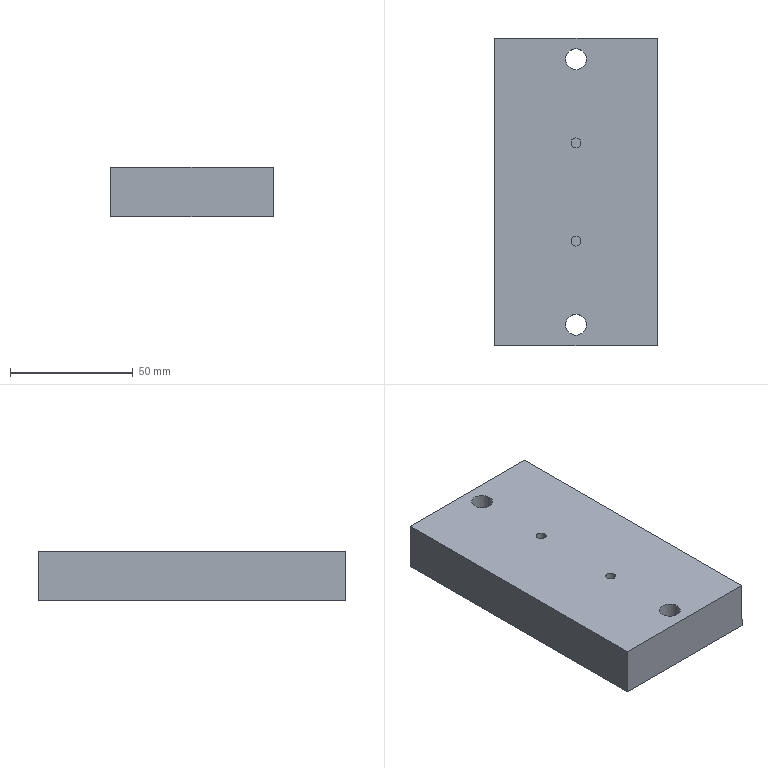NC program | NX | posted with a generic post | part box 65.936 x 125 x 20 mm
Lines 1209 to 2027 of 29196:
(PLANAR_MILL_1 , TOOL : D3R0)
N2308 T07 M6
N2310 G54
N2312 G17 G0 G90 X-29.604 Y-6.011 S5000 M3
N2314 G43 Z26.573 H7
N2316 G94 G1 Z-3.127 F5000.
N2318 X-29.572 Y-5.956 Z-3.128 F1000.
N2320 X-29.545 Y-5.795 Z-3.131
N2322 X-29.577 Y-5.636 Z-3.134
N2324 X-29.644 Y-5.519 Z-3.136
N2326 X-29.766 Y-5.412 Z-3.139
N2328 X-29.919 Y-5.355 Z-3.142
N2330 X-30.081 Z-3.145
N2332 X-30.234 Y-5.412 Z-3.148
N2334 X-30.356 Y-5.519 Z-3.151
N2336 X-30.423 Y-5.636 Z-3.153
N2338 X-30.45 Y-5.735 Z-3.155
N2340 Y-5.87 Z-3.157
N2342 X-30.406 Y-6.007 Z-3.16
N2344 X-30.322 Y-6.124 Z-3.162
N2346 X-30.205 Y-6.209 Z-3.165
N2348 X-30.067 Y-6.252 Z-3.167
N2350 X-29.933 Z-3.169
N2352 X-29.779 Y-6.2 Z-3.172
N2354 X-29.653 Y-6.097 Z-3.175
N2356 X-29.572 Y-5.956 Z-3.178
N2358 X-29.545 Y-5.795 Z-3.181
N2360 X-29.577 Y-5.636 Z-3.184
N2362 X-29.644 Y-5.519 Z-3.186
N2364 X-29.766 Y-5.412 Z-3.189
N2366 X-29.919 Y-5.355 Z-3.192
N2368 X-30.081 Z-3.195
N2370 X-30.234 Y-5.412 Z-3.197
N2372 X-30.356 Y-5.519 Z-3.2
N2374 X-30.423 Y-5.636 Z-3.203
N2376 X-30.45 Y-5.735 Z-3.204
N2378 Y-5.87 Z-3.207
N2380 X-30.406 Y-6.007 Z-3.209
N2382 X-30.322 Y-6.124 Z-3.212
N2384 X-30.205 Y-6.209 Z-3.214
N2386 X-30.067 Y-6.252 Z-3.217
N2388 X-29.933 Z-3.219
N2390 X-29.779 Y-6.2 Z-3.222
N2392 X-29.653 Y-6.097 Z-3.225
N2394 X-29.572 Y-5.956 Z-3.228
N2396 X-29.545 Y-5.795 Z-3.23
N2398 X-29.577 Y-5.636 Z-3.233
N2400 X-29.644 Y-5.519 Z-3.236
N2402 X-29.766 Y-5.412 Z-3.238
N2404 X-29.919 Y-5.355 Z-3.241
N2406 X-30.081 Z-3.244
N2408 X-30.234 Y-5.412 Z-3.247
N2410 X-30.356 Y-5.519 Z-3.25
N2412 X-30.423 Y-5.636 Z-3.252
N2414 X-30.45 Y-5.735 Z-3.254
N2416 Y-5.87 Z-3.256
N2418 X-30.406 Y-6.007 Z-3.259
N2420 X-30.322 Y-6.124 Z-3.261
N2422 X-30.205 Y-6.209 Z-3.264
N2424 X-30.067 Y-6.252 Z-3.266
N2426 X-29.933 Z-3.269
N2428 X-29.779 Y-6.2 Z-3.272
N2430 X-29.653 Y-6.097 Z-3.274
N2432 X-29.572 Y-5.956 Z-3.277
N2434 X-29.545 Y-5.795 Z-3.28
N2436 X-29.577 Y-5.636 Z-3.283
N2438 X-29.644 Y-5.519 Z-3.285
N2440 X-29.766 Y-5.412 Z-3.288
N2442 X-29.919 Y-5.355 Z-3.291
N2444 X-30.081 Z-3.294
N2446 X-30.234 Y-5.412 Z-3.297
N2448 X-30.356 Y-5.519 Z-3.3
N2450 X-30.423 Y-5.636 Z-3.302
N2452 X-30.45 Y-5.735 Z-3.304
N2454 Y-5.87 Z-3.306
N2456 X-30.406 Y-6.007 Z-3.309
N2458 X-30.322 Y-6.124 Z-3.311
N2460 X-30.205 Y-6.209 Z-3.314
N2462 X-30.067 Y-6.252 Z-3.316
N2464 X-29.933 Z-3.318
N2466 X-29.779 Y-6.2 Z-3.321
N2468 X-29.653 Y-6.097 Z-3.324
N2470 X-29.572 Y-5.956 Z-3.327
N2472 X-29.545 Y-5.795 Z-3.33
N2474 X-29.577 Y-5.636 Z-3.333
N2476 X-29.644 Y-5.519 Z-3.335
N2478 X-29.766 Y-5.412 Z-3.338
N2480 X-29.919 Y-5.355 Z-3.341
N2482 X-30.081 Z-3.344
N2484 X-30.234 Y-5.412 Z-3.346
N2486 X-30.356 Y-5.519 Z-3.349
N2488 X-30.423 Y-5.636 Z-3.352
N2490 X-30.45 Y-5.735 Z-3.353
N2492 Y-5.87 Z-3.356
N2494 X-30.406 Y-6.007 Z-3.358
N2496 X-30.322 Y-6.124 Z-3.361
N2498 X-30.205 Y-6.209 Z-3.363
N2500 X-30.067 Y-6.252 Z-3.366
N2502 X-29.933 Z-3.368
N2504 X-29.779 Y-6.2 Z-3.371
N2506 X-29.653 Y-6.097 Z-3.374
N2508 X-29.572 Y-5.956 Z-3.377
N2510 X-29.545 Y-5.795 Z-3.379
N2512 X-29.577 Y-5.636 Z-3.382
N2514 X-29.644 Y-5.519 Z-3.385
N2516 X-29.766 Y-5.412 Z-3.387
N2518 X-29.919 Y-5.355 Z-3.39
N2520 X-30.081 Z-3.393
N2522 X-30.234 Y-5.412 Z-3.396
N2524 X-30.356 Y-5.519 Z-3.399
N2526 X-30.423 Y-5.636 Z-3.401
N2528 X-30.45 Y-5.735 Z-3.403
N2530 Y-5.87 Z-3.405
N2532 X-30.406 Y-6.007 Z-3.408
N2534 X-30.322 Y-6.124 Z-3.41
N2536 X-30.205 Y-6.209 Z-3.413
N2538 X-30.067 Y-6.252 Z-3.415
N2540 X-29.933 Z-3.418
N2542 X-29.779 Y-6.2 Z-3.421
N2544 X-29.653 Y-6.097 Z-3.423
N2546 X-29.572 Y-5.956 Z-3.426
N2548 X-29.545 Y-5.795 Z-3.429
N2550 X-29.577 Y-5.636 Z-3.432
N2552 X-29.644 Y-5.519 Z-3.434
N2554 X-29.766 Y-5.412 Z-3.437
N2556 X-29.919 Y-5.355 Z-3.44
N2558 X-30.081 Z-3.443
N2560 X-30.234 Y-5.412 Z-3.446
N2562 X-30.356 Y-5.519 Z-3.449
N2564 X-30.423 Y-5.636 Z-3.451
N2566 X-30.45 Y-5.735 Z-3.453
N2568 Y-5.87 Z-3.455
N2570 X-30.406 Y-6.007 Z-3.458
N2572 X-30.322 Y-6.124 Z-3.46
N2574 X-30.205 Y-6.209 Z-3.463
N2576 X-30.067 Y-6.252 Z-3.465
N2578 X-29.933 Z-3.467
N2580 X-29.779 Y-6.2 Z-3.47
N2582 X-29.653 Y-6.097 Z-3.473
N2584 X-29.572 Y-5.956 Z-3.476
N2586 X-29.545 Y-5.795 Z-3.479
N2588 X-29.577 Y-5.636 Z-3.482
N2590 X-29.644 Y-5.519 Z-3.484
N2592 X-29.766 Y-5.412 Z-3.487
N2594 X-29.919 Y-5.355 Z-3.49
N2596 X-30.081 Z-3.493
N2598 X-30.234 Y-5.412 Z-3.495
N2600 X-30.356 Y-5.519 Z-3.498
N2602 X-30.423 Y-5.636 Z-3.501
N2604 X-30.45 Y-5.735 Z-3.502
N2606 Y-5.87 Z-3.505
N2608 X-30.406 Y-6.007 Z-3.507
N2610 X-30.322 Y-6.124 Z-3.51
N2612 X-30.205 Y-6.209 Z-3.512
N2614 X-30.067 Y-6.252 Z-3.515
N2616 X-29.933 Z-3.517
N2618 X-29.779 Y-6.2 Z-3.52
N2620 X-29.653 Y-6.097 Z-3.523
N2622 X-29.572 Y-5.956 Z-3.526
N2624 X-29.545 Y-5.795 Z-3.528
N2626 X-29.577 Y-5.636 Z-3.531
N2628 X-29.644 Y-5.519 Z-3.534
N2630 X-29.766 Y-5.412 Z-3.536
N2632 X-29.919 Y-5.355 Z-3.539
N2634 X-30.081 Z-3.542
N2636 X-30.234 Y-5.412 Z-3.545
N2638 X-30.356 Y-5.519 Z-3.548
N2640 X-30.423 Y-5.636 Z-3.55
N2642 X-30.45 Y-5.735 Z-3.552
N2644 Y-5.87 Z-3.554
N2646 X-30.406 Y-6.007 Z-3.557
N2648 X-30.322 Y-6.124 Z-3.559
N2650 X-30.205 Y-6.209 Z-3.562
N2652 X-30.067 Y-6.252 Z-3.564
N2654 X-29.933 Z-3.567
N2656 X-29.779 Y-6.2 Z-3.57
N2658 X-29.653 Y-6.097 Z-3.572
N2660 X-29.572 Y-5.956 Z-3.575
N2662 X-29.545 Y-5.795 Z-3.578
N2664 X-29.577 Y-5.636 Z-3.581
N2666 X-29.644 Y-5.519 Z-3.583
N2668 X-29.766 Y-5.412 Z-3.586
N2670 X-29.919 Y-5.355 Z-3.589
N2672 X-30.081 Z-3.592
N2674 X-30.234 Y-5.412 Z-3.595
N2676 X-30.356 Y-5.519 Z-3.598
N2678 X-30.423 Y-5.636 Z-3.6
N2680 X-30.45 Y-5.735 Z-3.602
N2682 Y-5.87 Z-3.604
N2684 X-30.406 Y-6.007 Z-3.607
N2686 X-30.322 Y-6.124 Z-3.609
N2688 X-30.205 Y-6.209 Z-3.612
N2690 X-30.067 Y-6.252 Z-3.614
N2692 X-29.933 Z-3.616
N2694 X-29.779 Y-6.2 Z-3.619
N2696 X-29.653 Y-6.097 Z-3.622
N2698 X-29.572 Y-5.956 Z-3.625
N2700 X-29.545 Y-5.795 Z-3.628
N2702 X-29.577 Y-5.636 Z-3.631
N2704 X-29.644 Y-5.519 Z-3.633
N2706 X-29.766 Y-5.412 Z-3.636
N2708 X-29.919 Y-5.355 Z-3.639
N2710 X-30.081 Z-3.642
N2712 X-30.234 Y-5.412 Z-3.644
N2714 X-30.356 Y-5.519 Z-3.647
N2716 X-30.423 Y-5.636 Z-3.65
N2718 X-30.45 Y-5.735 Z-3.651
N2720 Y-5.87 Z-3.654
N2722 X-30.406 Y-6.007 Z-3.656
N2724 X-30.322 Y-6.124 Z-3.659
N2726 X-30.205 Y-6.209 Z-3.661
N2728 X-30.067 Y-6.252 Z-3.664
N2730 X-29.933 Z-3.666
N2732 X-29.779 Y-6.2 Z-3.669
N2734 X-29.653 Y-6.097 Z-3.672
N2736 X-29.572 Y-5.956 Z-3.675
N2738 X-29.545 Y-5.795 Z-3.677
N2740 X-29.577 Y-5.636 Z-3.68
N2742 X-29.644 Y-5.519 Z-3.683
N2744 X-29.766 Y-5.412 Z-3.685
N2746 X-29.919 Y-5.355 Z-3.688
N2748 X-30.081 Z-3.691
N2750 X-30.234 Y-5.412 Z-3.694
N2752 X-30.356 Y-5.519 Z-3.697
N2754 X-30.423 Y-5.636 Z-3.699
N2756 X-30.45 Y-5.735 Z-3.701
N2758 Y-5.87 Z-3.703
N2760 X-30.406 Y-6.007 Z-3.706
N2762 X-30.322 Y-6.124 Z-3.708
N2764 X-30.205 Y-6.209 Z-3.711
N2766 X-30.067 Y-6.252 Z-3.713
N2768 X-29.933 Z-3.716
N2770 X-29.779 Y-6.2 Z-3.719
N2772 X-29.653 Y-6.097 Z-3.721
N2774 X-29.572 Y-5.956 Z-3.724
N2776 X-29.545 Y-5.795 Z-3.727
N2778 X-29.577 Y-5.636 Z-3.73
N2780 X-29.644 Y-5.519 Z-3.732
N2782 X-29.766 Y-5.412 Z-3.735
N2784 X-29.919 Y-5.355 Z-3.738
N2786 X-30.081 Z-3.741
N2788 X-30.234 Y-5.412 Z-3.744
N2790 X-30.356 Y-5.519 Z-3.747
N2792 X-30.423 Y-5.636 Z-3.749
N2794 X-30.45 Y-5.735 Z-3.751
N2796 Y-5.87 Z-3.753
N2798 X-30.406 Y-6.007 Z-3.756
N2800 X-30.322 Y-6.124 Z-3.758
N2802 X-30.205 Y-6.209 Z-3.761
N2804 X-30.067 Y-6.252 Z-3.763
N2806 X-29.933 Z-3.765
N2808 X-29.779 Y-6.2 Z-3.768
N2810 X-29.653 Y-6.097 Z-3.771
N2812 X-29.572 Y-5.956 Z-3.774
N2814 X-29.545 Y-5.795 Z-3.777
N2816 X-29.577 Y-5.636 Z-3.78
N2818 X-29.644 Y-5.519 Z-3.782
N2820 X-29.766 Y-5.412 Z-3.785
N2822 X-29.919 Y-5.355 Z-3.788
N2824 X-30.081 Z-3.791
N2826 X-30.234 Y-5.412 Z-3.793
N2828 X-30.356 Y-5.519 Z-3.796
N2830 X-30.423 Y-5.636 Z-3.799
N2832 X-30.45 Y-5.735 Z-3.8
N2834 Y-5.87 Z-3.803
N2836 X-30.406 Y-6.007 Z-3.805
N2838 X-30.322 Y-6.124 Z-3.808
N2840 X-30.205 Y-6.209 Z-3.81
N2842 X-30.067 Y-6.252 Z-3.813
N2844 X-29.933 Z-3.815
N2846 X-29.779 Y-6.2 Z-3.818
N2848 X-29.653 Y-6.097 Z-3.821
N2850 X-29.572 Y-5.956 Z-3.824
N2852 X-29.545 Y-5.795 Z-3.826
N2854 X-29.577 Y-5.636 Z-3.829
N2856 X-29.644 Y-5.519 Z-3.832
N2858 X-29.766 Y-5.412 Z-3.834
N2860 X-29.919 Y-5.355 Z-3.837
N2862 X-30.081 Z-3.84
N2864 X-30.234 Y-5.412 Z-3.843
N2866 X-30.356 Y-5.519 Z-3.846
N2868 X-30.423 Y-5.636 Z-3.848
N2870 X-30.45 Y-5.735 Z-3.85
N2872 Y-5.87 Z-3.852
N2874 X-30.406 Y-6.007 Z-3.855
N2876 X-30.322 Y-6.124 Z-3.857
N2878 X-30.205 Y-6.209 Z-3.86
N2880 X-30.067 Y-6.252 Z-3.862
N2882 X-29.933 Z-3.865
N2884 X-29.779 Y-6.2 Z-3.868
N2886 X-29.653 Y-6.097 Z-3.87
N2888 X-29.572 Y-5.956 Z-3.873
N2890 X-29.545 Y-5.795 Z-3.876
N2892 X-29.577 Y-5.636 Z-3.879
N2894 X-29.644 Y-5.519 Z-3.881
N2896 X-29.766 Y-5.412 Z-3.884
N2898 X-29.919 Y-5.355 Z-3.887
N2900 X-30.081 Z-3.89
N2902 X-30.234 Y-5.412 Z-3.893
N2904 X-30.356 Y-5.519 Z-3.896
N2906 X-30.423 Y-5.636 Z-3.898
N2908 X-30.45 Y-5.735 Z-3.9
N2910 Y-5.87 Z-3.902
N2912 X-30.406 Y-6.007 Z-3.905
N2914 X-30.322 Y-6.124 Z-3.907
N2916 X-30.205 Y-6.209 Z-3.91
N2918 X-30.067 Y-6.252 Z-3.912
N2920 X-29.933 Z-3.914
N2922 X-29.779 Y-6.2 Z-3.917
N2924 X-29.653 Y-6.097 Z-3.92
N2926 X-29.572 Y-5.956 Z-3.923
N2928 X-29.545 Y-5.795 Z-3.926
N2930 X-29.577 Y-5.636 Z-3.929
N2932 X-29.644 Y-5.519 Z-3.931
N2934 X-29.766 Y-5.412 Z-3.934
N2936 X-29.919 Y-5.355 Z-3.937
N2938 X-30.081 Z-3.94
N2940 X-30.234 Y-5.412 Z-3.942
N2942 X-30.356 Y-5.519 Z-3.945
N2944 X-30.423 Y-5.636 Z-3.948
N2946 X-30.45 Y-5.735 Z-3.949
N2948 Y-5.87 Z-3.952
N2950 X-30.406 Y-6.007 Z-3.954
N2952 X-30.322 Y-6.124 Z-3.957
N2954 X-30.205 Y-6.209 Z-3.959
N2956 X-30.067 Y-6.252 Z-3.962
N2958 X-29.933 Z-3.964
N2960 X-29.779 Y-6.2 Z-3.967
N2962 X-29.653 Y-6.097 Z-3.97
N2964 X-29.572 Y-5.956 Z-3.973
N2966 X-29.545 Y-5.795 Z-3.975
N2968 X-29.577 Y-5.636 Z-3.978
N2970 X-29.644 Y-5.519 Z-3.981
N2972 X-29.766 Y-5.412 Z-3.983
N2974 X-29.919 Y-5.355 Z-3.986
N2976 X-30.081 Z-3.989
N2978 X-30.234 Y-5.412 Z-3.992
N2980 X-30.356 Y-5.519 Z-3.995
N2982 X-30.423 Y-5.636 Z-3.997
N2984 X-30.45 Y-5.735 Z-3.999
N2986 Y-5.87 Z-4.001
N2988 X-30.406 Y-6.007 Z-4.004
N2990 X-30.322 Y-6.124 Z-4.006
N2992 X-30.205 Y-6.209 Z-4.009
N2994 X-30.067 Y-6.252 Z-4.011
N2996 X-29.933 Z-4.014
N2998 X-29.779 Y-6.2 Z-4.017
N3000 X-29.653 Y-6.097 Z-4.019
N3002 X-29.572 Y-5.956 Z-4.022
N3004 X-29.545 Y-5.795 Z-4.025
N3006 X-29.577 Y-5.636 Z-4.028
N3008 X-29.644 Y-5.519 Z-4.03
N3010 X-29.766 Y-5.412 Z-4.033
N3012 X-29.919 Y-5.355 Z-4.036
N3014 X-30.081 Z-4.039
N3016 X-30.234 Y-5.412 Z-4.042
N3018 X-30.356 Y-5.519 Z-4.045
N3020 X-30.423 Y-5.636 Z-4.047
N3022 X-30.45 Y-5.735 Z-4.049
N3024 Y-5.87 Z-4.051
N3026 X-30.406 Y-6.007 Z-4.054
N3028 X-30.322 Y-6.124 Z-4.056
N3030 X-30.205 Y-6.209 Z-4.059
N3032 X-30.067 Y-6.252 Z-4.061
N3034 X-29.933 Z-4.063
N3036 X-29.779 Y-6.2 Z-4.066
N3038 X-29.653 Y-6.097 Z-4.069
N3040 X-29.572 Y-5.956 Z-4.072
N3042 X-29.545 Y-5.795 Z-4.075
N3044 X-29.577 Y-5.636 Z-4.078
N3046 X-29.644 Y-5.519 Z-4.08
N3048 X-29.766 Y-5.412 Z-4.083
N3050 X-29.919 Y-5.355 Z-4.086
N3052 X-30.081 Z-4.089
N3054 X-30.234 Y-5.412 Z-4.091
N3056 X-30.356 Y-5.519 Z-4.094
N3058 X-30.423 Y-5.636 Z-4.097
N3060 X-30.45 Y-5.735 Z-4.098
N3062 Y-5.87 Z-4.101
N3064 X-30.406 Y-6.007 Z-4.103
N3066 X-30.322 Y-6.124 Z-4.106
N3068 X-30.205 Y-6.209 Z-4.108
N3070 X-30.067 Y-6.252 Z-4.111
N3072 X-29.933 Z-4.113
N3074 X-29.779 Y-6.2 Z-4.116
N3076 X-29.653 Y-6.097 Z-4.119
N3078 X-29.572 Y-5.956 Z-4.122
N3080 X-29.545 Y-5.795 Z-4.124
N3082 X-29.577 Y-5.636 Z-4.127
N3084 X-29.644 Y-5.519 Z-4.13
N3086 X-29.766 Y-5.412 Z-4.132
N3088 X-29.919 Y-5.355 Z-4.135
N3090 X-30.081 Z-4.138
N3092 X-30.234 Y-5.412 Z-4.141
N3094 X-30.356 Y-5.519 Z-4.144
N3096 X-30.423 Y-5.636 Z-4.146
N3098 X-30.45 Y-5.735 Z-4.148
N3100 Y-5.87 Z-4.15
N3102 X-30.406 Y-6.007 Z-4.153
N3104 X-30.322 Y-6.124 Z-4.155
N3106 X-30.205 Y-6.209 Z-4.158
N3108 X-30.067 Y-6.252 Z-4.16
N3110 X-29.933 Z-4.163
N3112 X-29.779 Y-6.2 Z-4.166
N3114 X-29.653 Y-6.097 Z-4.168
N3116 X-29.572 Y-5.956 Z-4.171
N3118 X-29.545 Y-5.795 Z-4.174
N3120 X-29.577 Y-5.636 Z-4.177
N3122 X-29.644 Y-5.519 Z-4.179
N3124 X-29.766 Y-5.412 Z-4.182
N3126 X-29.919 Y-5.355 Z-4.185
N3128 X-30.081 Z-4.188
N3130 X-30.234 Y-5.412 Z-4.191
N3132 X-30.356 Y-5.519 Z-4.194
N3134 X-30.423 Y-5.636 Z-4.196
N3136 X-30.45 Y-5.735 Z-4.198
N3138 Y-5.87 Z-4.2
N3140 X-30.406 Y-6.007 Z-4.203
N3142 X-30.322 Y-6.124 Z-4.205
N3144 X-30.205 Y-6.209 Z-4.208
N3146 X-30.067 Y-6.252 Z-4.21
N3148 X-29.933 Z-4.212
N3150 X-29.779 Y-6.2 Z-4.215
N3152 X-29.653 Y-6.097 Z-4.218
N3154 X-29.572 Y-5.956 Z-4.221
N3156 X-29.545 Y-5.795 Z-4.224
N3158 X-29.577 Y-5.636 Z-4.227
N3160 X-29.644 Y-5.519 Z-4.229
N3162 X-29.766 Y-5.412 Z-4.232
N3164 X-29.919 Y-5.355 Z-4.235
N3166 X-30.081 Z-4.238
N3168 X-30.234 Y-5.412 Z-4.24
N3170 X-30.356 Y-5.519 Z-4.243
N3172 X-30.423 Y-5.636 Z-4.246
N3174 X-30.45 Y-5.735 Z-4.247
N3176 Y-5.87 Z-4.25
N3178 X-30.406 Y-6.007 Z-4.252
N3180 X-30.322 Y-6.124 Z-4.255
N3182 X-30.205 Y-6.209 Z-4.257
N3184 X-30.067 Y-6.252 Z-4.26
N3186 X-29.933 Z-4.262
N3188 X-29.779 Y-6.2 Z-4.265
N3190 X-29.653 Y-6.097 Z-4.268
N3192 X-29.572 Y-5.956 Z-4.271
N3194 X-29.545 Y-5.795 Z-4.273
N3196 X-29.577 Y-5.636 Z-4.276
N3198 X-29.644 Y-5.519 Z-4.279
N3200 X-29.766 Y-5.412 Z-4.281
N3202 X-29.919 Y-5.355 Z-4.284
N3204 X-30.081 Z-4.287
N3206 X-30.234 Y-5.412 Z-4.29
N3208 X-30.356 Y-5.519 Z-4.293
N3210 X-30.423 Y-5.636 Z-4.295
N3212 X-30.45 Y-5.735 Z-4.297
N3214 Y-5.87 Z-4.299
N3216 X-30.406 Y-6.007 Z-4.302
N3218 X-30.322 Y-6.124 Z-4.304
N3220 X-30.205 Y-6.209 Z-4.307
N3222 X-30.067 Y-6.252 Z-4.309
N3224 X-29.933 Z-4.312
N3226 X-29.779 Y-6.2 Z-4.315
N3228 X-29.653 Y-6.097 Z-4.317
N3230 X-29.572 Y-5.956 Z-4.32
N3232 X-29.545 Y-5.795 Z-4.323
N3234 X-29.577 Y-5.636 Z-4.326
N3236 X-29.644 Y-5.519 Z-4.328
N3238 X-29.766 Y-5.412 Z-4.331
N3240 X-29.919 Y-5.355 Z-4.334
N3242 X-30.081 Z-4.337
N3244 X-30.234 Y-5.412 Z-4.34
N3246 X-30.356 Y-5.519 Z-4.343
N3248 X-30.423 Y-5.636 Z-4.345
N3250 X-30.45 Y-5.735 Z-4.347
N3252 Y-5.87 Z-4.349
N3254 X-30.406 Y-6.007 Z-4.352
N3256 X-30.322 Y-6.124 Z-4.354
N3258 X-30.205 Y-6.209 Z-4.357
N3260 X-30.067 Y-6.252 Z-4.359
N3262 X-29.933 Z-4.361
N3264 X-29.779 Y-6.2 Z-4.364
N3266 X-29.653 Y-6.097 Z-4.367
N3268 X-29.572 Y-5.956 Z-4.37
N3270 X-29.545 Y-5.795 Z-4.373
N3272 X-29.577 Y-5.636 Z-4.376
N3274 X-29.644 Y-5.519 Z-4.378
N3276 X-29.766 Y-5.412 Z-4.381
N3278 X-29.919 Y-5.355 Z-4.384
N3280 X-30.081 Z-4.387
N3282 X-30.234 Y-5.412 Z-4.389
N3284 X-30.356 Y-5.519 Z-4.392
N3286 X-30.423 Y-5.636 Z-4.395
N3288 X-30.45 Y-5.735 Z-4.396
N3290 Y-5.87 Z-4.399
N3292 X-30.406 Y-6.007 Z-4.401
N3294 X-30.322 Y-6.124 Z-4.404
N3296 X-30.205 Y-6.209 Z-4.406
N3298 X-30.067 Y-6.252 Z-4.409
N3300 X-29.933 Z-4.411
N3302 X-29.779 Y-6.2 Z-4.414
N3304 X-29.653 Y-6.097 Z-4.417
N3306 X-29.572 Y-5.956 Z-4.42
N3308 X-29.545 Y-5.795 Z-4.422
N3310 X-29.577 Y-5.636 Z-4.425
N3312 X-29.644 Y-5.519 Z-4.428
N3314 X-29.766 Y-5.412 Z-4.43
N3316 X-29.919 Y-5.355 Z-4.433
N3318 X-30.081 Z-4.436
N3320 X-30.234 Y-5.412 Z-4.439
N3322 X-30.356 Y-5.519 Z-4.442
N3324 X-30.423 Y-5.636 Z-4.444
N3326 X-30.45 Y-5.735 Z-4.446
N3328 Y-5.87 Z-4.448
N3330 X-30.406 Y-6.007 Z-4.451
N3332 X-30.322 Y-6.124 Z-4.453
N3334 X-30.205 Y-6.209 Z-4.456
N3336 X-30.067 Y-6.252 Z-4.458
N3338 X-29.933 Z-4.461
N3340 X-29.779 Y-6.2 Z-4.464
N3342 X-29.653 Y-6.097 Z-4.466
N3344 X-29.572 Y-5.956 Z-4.469
N3346 X-29.545 Y-5.795 Z-4.472
N3348 X-29.577 Y-5.636 Z-4.475
N3350 X-29.644 Y-5.519 Z-4.477
N3352 X-29.766 Y-5.412 Z-4.48
N3354 X-29.919 Y-5.355 Z-4.483
N3356 X-30.081 Z-4.486
N3358 X-30.234 Y-5.412 Z-4.489
N3360 X-30.356 Y-5.519 Z-4.492
N3362 X-30.423 Y-5.636 Z-4.494
N3364 X-30.45 Y-5.735 Z-4.496
N3366 Y-5.87 Z-4.498
N3368 X-30.406 Y-6.007 Z-4.501
N3370 X-30.322 Y-6.124 Z-4.503
N3372 X-30.205 Y-6.209 Z-4.506
N3374 X-30.067 Y-6.252 Z-4.508
N3376 X-29.933 Z-4.51
N3378 X-29.779 Y-6.2 Z-4.513
N3380 X-29.653 Y-6.097 Z-4.516
N3382 X-29.572 Y-5.956 Z-4.519
N3384 X-29.545 Y-5.795 Z-4.522
N3386 X-29.577 Y-5.636 Z-4.525
N3388 X-29.644 Y-5.519 Z-4.527
N3390 X-29.766 Y-5.412 Z-4.53
N3392 X-29.919 Y-5.355 Z-4.533
N3394 X-30.081 Z-4.536
N3396 X-30.234 Y-5.412 Z-4.538
N3398 X-30.356 Y-5.519 Z-4.541
N3400 X-30.423 Y-5.636 Z-4.544
N3402 X-30.45 Y-5.735 Z-4.545
N3404 Y-5.87 Z-4.548
N3406 X-30.406 Y-6.007 Z-4.55
N3408 X-30.322 Y-6.124 Z-4.553
N3410 X-30.205 Y-6.209 Z-4.555
N3412 X-30.067 Y-6.252 Z-4.558
N3414 X-29.933 Z-4.56
N3416 X-29.779 Y-6.2 Z-4.563
N3418 X-29.653 Y-6.097 Z-4.566
N3420 X-29.572 Y-5.956 Z-4.569
N3422 X-29.545 Y-5.795 Z-4.571
N3424 X-29.577 Y-5.636 Z-4.574
N3426 X-29.644 Y-5.519 Z-4.577
N3428 X-29.766 Y-5.412 Z-4.579
N3430 X-29.919 Y-5.355 Z-4.582
N3432 X-30.081 Z-4.585
N3434 X-30.234 Y-5.412 Z-4.588
N3436 X-30.356 Y-5.519 Z-4.591
N3438 X-30.423 Y-5.636 Z-4.593
N3440 X-30.45 Y-5.735 Z-4.595
N3442 Y-5.87 Z-4.597
N3444 X-30.406 Y-6.007 Z-4.6
N3446 X-30.322 Y-6.124 Z-4.602
N3448 X-30.205 Y-6.209 Z-4.605
N3450 X-30.067 Y-6.252 Z-4.607
N3452 X-29.933 Z-4.61
N3454 X-29.779 Y-6.2 Z-4.613
N3456 X-29.653 Y-6.097 Z-4.615
N3458 X-29.572 Y-5.956 Z-4.618
N3460 X-29.545 Y-5.795 Z-4.621
N3462 X-29.577 Y-5.636 Z-4.624
N3464 X-29.644 Y-5.519 Z-4.626
N3466 X-29.766 Y-5.412 Z-4.629
N3468 X-29.919 Y-5.355 Z-4.632
N3470 X-30.081 Z-4.635
N3472 X-30.234 Y-5.412 Z-4.638
N3474 X-30.356 Y-5.519 Z-4.641
N3476 X-30.423 Y-5.636 Z-4.643
N3478 X-30.45 Y-5.735 Z-4.645
N3480 Y-5.87 Z-4.647
N3482 X-30.406 Y-6.007 Z-4.65
N3484 X-30.322 Y-6.124 Z-4.652
N3486 X-30.205 Y-6.209 Z-4.655
N3488 X-30.067 Y-6.252 Z-4.657
N3490 X-29.933 Z-4.659
N3492 X-29.779 Y-6.2 Z-4.662
N3494 X-29.653 Y-6.097 Z-4.665
N3496 X-29.572 Y-5.956 Z-4.668
N3498 X-29.545 Y-5.795 Z-4.671
N3500 X-29.577 Y-5.636 Z-4.674
N3502 X-29.644 Y-5.519 Z-4.676
N3504 X-29.766 Y-5.412 Z-4.679
N3506 X-29.919 Y-5.355 Z-4.682
N3508 X-30.081 Z-4.685
N3510 X-30.234 Y-5.412 Z-4.687
N3512 X-30.356 Y-5.519 Z-4.69
N3514 X-30.423 Y-5.636 Z-4.693
N3516 X-30.45 Y-5.735 Z-4.694
N3518 Y-5.87 Z-4.697
N3520 X-30.406 Y-6.007 Z-4.699
N3522 X-30.322 Y-6.124 Z-4.702
N3524 X-30.205 Y-6.209 Z-4.704
N3526 X-30.067 Y-6.252 Z-4.707
N3528 X-29.933 Z-4.709
N3530 X-29.779 Y-6.2 Z-4.712
N3532 X-29.653 Y-6.097 Z-4.715
N3534 X-29.572 Y-5.956 Z-4.718
N3536 X-29.545 Y-5.795 Z-4.72
N3538 X-29.577 Y-5.636 Z-4.723
N3540 X-29.644 Y-5.519 Z-4.726
N3542 X-29.766 Y-5.412 Z-4.728
N3544 X-29.919 Y-5.355 Z-4.731
N3546 X-30.081 Z-4.734
N3548 X-30.234 Y-5.412 Z-4.737
N3550 X-30.356 Y-5.519 Z-4.74
N3552 X-30.423 Y-5.636 Z-4.742
N3554 X-30.45 Y-5.735 Z-4.744
N3556 Y-5.87 Z-4.746
N3558 X-30.406 Y-6.007 Z-4.749
N3560 X-30.322 Y-6.124 Z-4.751
N3562 X-30.205 Y-6.209 Z-4.754
N3564 X-30.067 Y-6.252 Z-4.756
N3566 X-29.933 Z-4.759
N3568 X-29.779 Y-6.2 Z-4.762
N3570 X-29.653 Y-6.097 Z-4.764
N3572 X-29.572 Y-5.956 Z-4.767
N3574 X-29.545 Y-5.795 Z-4.77
N3576 X-29.577 Y-5.636 Z-4.773
N3578 X-29.644 Y-5.519 Z-4.775
N3580 X-29.766 Y-5.412 Z-4.778
N3582 X-29.919 Y-5.355 Z-4.781
N3584 X-30.081 Z-4.784
N3586 X-30.234 Y-5.412 Z-4.787
N3588 X-30.356 Y-5.519 Z-4.79
N3590 X-30.423 Y-5.636 Z-4.792
N3592 X-30.45 Y-5.735 Z-4.794
N3594 Y-5.87 Z-4.796
N3596 X-30.406 Y-6.007 Z-4.799
N3598 X-30.322 Y-6.124 Z-4.801
N3600 X-30.205 Y-6.209 Z-4.804
N3602 X-30.067 Y-6.252 Z-4.806
N3604 X-29.933 Z-4.808
N3606 X-29.779 Y-6.2 Z-4.811
N3608 X-29.653 Y-6.097 Z-4.814
N3610 X-29.572 Y-5.956 Z-4.817
N3612 X-29.545 Y-5.795 Z-4.82
N3614 X-29.577 Y-5.636 Z-4.823
N3616 X-29.644 Y-5.519 Z-4.825
N3618 X-29.766 Y-5.412 Z-4.828
N3620 X-29.919 Y-5.355 Z-4.831
N3622 X-30.081 Z-4.834
N3624 X-30.234 Y-5.412 Z-4.836
N3626 X-30.356 Y-5.519 Z-4.839
N3628 X-30.423 Y-5.636 Z-4.842
N3630 X-30.45 Y-5.735 Z-4.843
N3632 Y-5.87 Z-4.846
N3634 X-30.406 Y-6.007 Z-4.848
N3636 X-30.322 Y-6.124 Z-4.851
N3638 X-30.205 Y-6.209 Z-4.853
N3640 X-30.067 Y-6.252 Z-4.856
N3642 X-29.933 Z-4.858
N3644 X-29.779 Y-6.2 Z-4.861
N3646 X-29.653 Y-6.097 Z-4.864
N3648 X-29.572 Y-5.956 Z-4.867
N3650 X-29.545 Y-5.795 Z-4.869
N3652 X-29.577 Y-5.636 Z-4.872
N3654 X-29.644 Y-5.519 Z-4.875
N3656 X-29.766 Y-5.412 Z-4.877
N3658 X-29.919 Y-5.355 Z-4.88
N3660 X-30.081 Z-4.883
N3662 X-30.234 Y-5.412 Z-4.886
N3664 X-30.356 Y-5.519 Z-4.889
N3666 X-30.423 Y-5.636 Z-4.891
N3668 X-30.45 Y-5.735 Z-4.893
N3670 Y-5.87 Z-4.895
N3672 X-30.406 Y-6.007 Z-4.898
N3674 X-30.322 Y-6.124 Z-4.9
N3676 X-30.205 Y-6.209 Z-4.903
N3678 X-30.067 Y-6.252 Z-4.905
N3680 X-29.933 Z-4.908
N3682 X-29.779 Y-6.2 Z-4.911
N3684 X-29.653 Y-6.097 Z-4.913
N3686 X-29.572 Y-5.956 Z-4.916
N3688 X-29.545 Y-5.795 Z-4.919
N3690 X-29.577 Y-5.636 Z-4.922
N3692 X-29.644 Y-5.519 Z-4.924
N3694 X-29.766 Y-5.412 Z-4.927
N3696 X-29.919 Y-5.355 Z-4.93
N3698 X-30.081 Z-4.933
N3700 X-30.234 Y-5.412 Z-4.936
N3702 X-30.356 Y-5.519 Z-4.939
N3704 X-30.423 Y-5.636 Z-4.941
N3706 X-30.45 Y-5.735 Z-4.943
N3708 Y-5.87 Z-4.945
N3710 X-30.406 Y-6.007 Z-4.948
N3712 X-30.322 Y-6.124 Z-4.95
N3714 X-30.205 Y-6.209 Z-4.953
N3716 X-30.067 Y-6.252 Z-4.955
N3718 X-29.933 Z-4.957
N3720 X-29.779 Y-6.2 Z-4.96
N3722 X-29.653 Y-6.097 Z-4.963
N3724 X-29.572 Y-5.956 Z-4.966
N3726 X-29.545 Y-5.795 Z-4.969
N3728 X-29.577 Y-5.636 Z-4.972
N3730 X-29.644 Y-5.519 Z-4.974
N3732 X-29.766 Y-5.412 Z-4.977
N3734 X-29.919 Y-5.355 Z-4.98
N3736 X-30.081 Z-4.983
N3738 X-30.234 Y-5.412 Z-4.985
N3740 X-30.356 Y-5.519 Z-4.988
N3742 X-30.423 Y-5.636 Z-4.991
N3744 X-30.45 Y-5.735 Z-4.992
N3746 Y-5.87 Z-4.995
N3748 X-30.406 Y-6.007 Z-4.997
N3750 X-30.322 Y-6.124 Z-5.
N3752 X-30.205 Y-6.209 Z-5.002
N3754 X-30.067 Y-6.252 Z-5.005
N3756 X-29.933 Z-5.007
N3758 X-29.779 Y-6.2 Z-5.01
N3760 X-29.653 Y-6.097 Z-5.013
N3762 X-29.572 Y-5.956 Z-5.016
N3764 X-29.545 Y-5.795 Z-5.018
N3766 X-29.577 Y-5.636 Z-5.021
N3768 X-29.644 Y-5.519 Z-5.024
N3770 X-29.766 Y-5.412 Z-5.026
N3772 X-29.919 Y-5.355 Z-5.029
N3774 X-30.081 Z-5.032
N3776 X-30.234 Y-5.412 Z-5.035
N3778 X-30.356 Y-5.519 Z-5.038
N3780 X-30.423 Y-5.636 Z-5.04
N3782 X-30.45 Y-5.735 Z-5.042
N3784 Y-5.87 Z-5.044
N3786 X-30.406 Y-6.007 Z-5.047
N3788 X-30.322 Y-6.124 Z-5.049
N3790 X-30.205 Y-6.209 Z-5.052
N3792 X-30.067 Y-6.252 Z-5.054
N3794 X-29.933 Z-5.057
N3796 X-29.779 Y-6.2 Z-5.06
N3798 X-29.653 Y-6.097 Z-5.062
N3800 X-29.572 Y-5.956 Z-5.065
N3802 X-29.545 Y-5.795 Z-5.068
N3804 X-29.577 Y-5.636 Z-5.071
N3806 X-29.644 Y-5.519 Z-5.073
N3808 X-29.766 Y-5.412 Z-5.076
N3810 X-29.919 Y-5.355 Z-5.079
N3812 X-30.081 Z-5.082
N3814 X-30.234 Y-5.412 Z-5.085
N3816 X-30.356 Y-5.519 Z-5.088
N3818 X-30.423 Y-5.636 Z-5.09
N3820 X-30.45 Y-5.735 Z-5.092
N3822 Y-5.87 Z-5.094
N3824 X-30.406 Y-6.007 Z-5.097
N3826 X-30.322 Y-6.124 Z-5.099
N3828 X-30.205 Y-6.209 Z-5.102
N3830 X-30.067 Y-6.252 Z-5.104
N3832 X-29.933 Z-5.106
N3834 X-29.779 Y-6.2 Z-5.109
N3836 X-29.653 Y-6.097 Z-5.112
N3838 X-29.572 Y-5.956 Z-5.115
N3840 X-29.545 Y-5.795 Z-5.118
N3842 X-29.577 Y-5.636 Z-5.121
N3844 X-29.644 Y-5.519 Z-5.123
N3846 X-29.766 Y-5.412 Z-5.126
N3848 X-29.919 Y-5.355 Z-5.129
N3850 X-30.081 Z-5.132
N3852 X-30.234 Y-5.412 Z-5.134
N3854 X-30.356 Y-5.519 Z-5.137
N3856 X-30.423 Y-5.636 Z-5.14
N3858 X-30.45 Y-5.735 Z-5.141
N3860 Y-5.87 Z-5.144
N3862 X-30.406 Y-6.007 Z-5.146
N3864 X-30.322 Y-6.124 Z-5.149
N3866 X-30.205 Y-6.209 Z-5.151
N3868 X-30.067 Y-6.252 Z-5.154
N3870 X-29.933 Z-5.156
N3872 X-29.779 Y-6.2 Z-5.159
N3874 X-29.653 Y-6.097 Z-5.162
N3876 X-29.572 Y-5.956 Z-5.165
N3878 X-29.545 Y-5.795 Z-5.167
N3880 X-29.577 Y-5.636 Z-5.17
N3882 X-29.644 Y-5.519 Z-5.173
N3884 X-29.766 Y-5.412 Z-5.175
N3886 X-29.919 Y-5.355 Z-5.178
N3888 X-30.081 Z-5.181
N3890 X-30.234 Y-5.412 Z-5.184
N3892 X-30.356 Y-5.519 Z-5.187
N3894 X-30.423 Y-5.636 Z-5.189
N3896 X-30.45 Y-5.735 Z-5.191
N3898 Y-5.87 Z-5.193
N3900 X-30.406 Y-6.007 Z-5.196
N3902 X-30.322 Y-6.124 Z-5.198
N3904 X-30.205 Y-6.209 Z-5.201
N3906 X-30.067 Y-6.252 Z-5.203
N3908 X-29.933 Z-5.206
N3910 X-29.779 Y-6.2 Z-5.209
N3912 X-29.653 Y-6.097 Z-5.211
N3914 X-29.572 Y-5.956 Z-5.214
N3916 X-29.545 Y-5.795 Z-5.217
N3918 X-29.577 Y-5.636 Z-5.22
N3920 X-29.644 Y-5.519 Z-5.222
N3922 X-29.766 Y-5.412 Z-5.225
N3924 X-29.919 Y-5.355 Z-5.228
N3926 X-30.081 Z-5.231
N3928 X-30.234 Y-5.412 Z-5.234
N3930 X-30.356 Y-5.519 Z-5.237
N3932 X-30.423 Y-5.636 Z-5.239
N3934 X-30.45 Y-5.735 Z-5.241
N3936 Y-5.87 Z-5.243
N3938 X-30.406 Y-6.007 Z-5.246